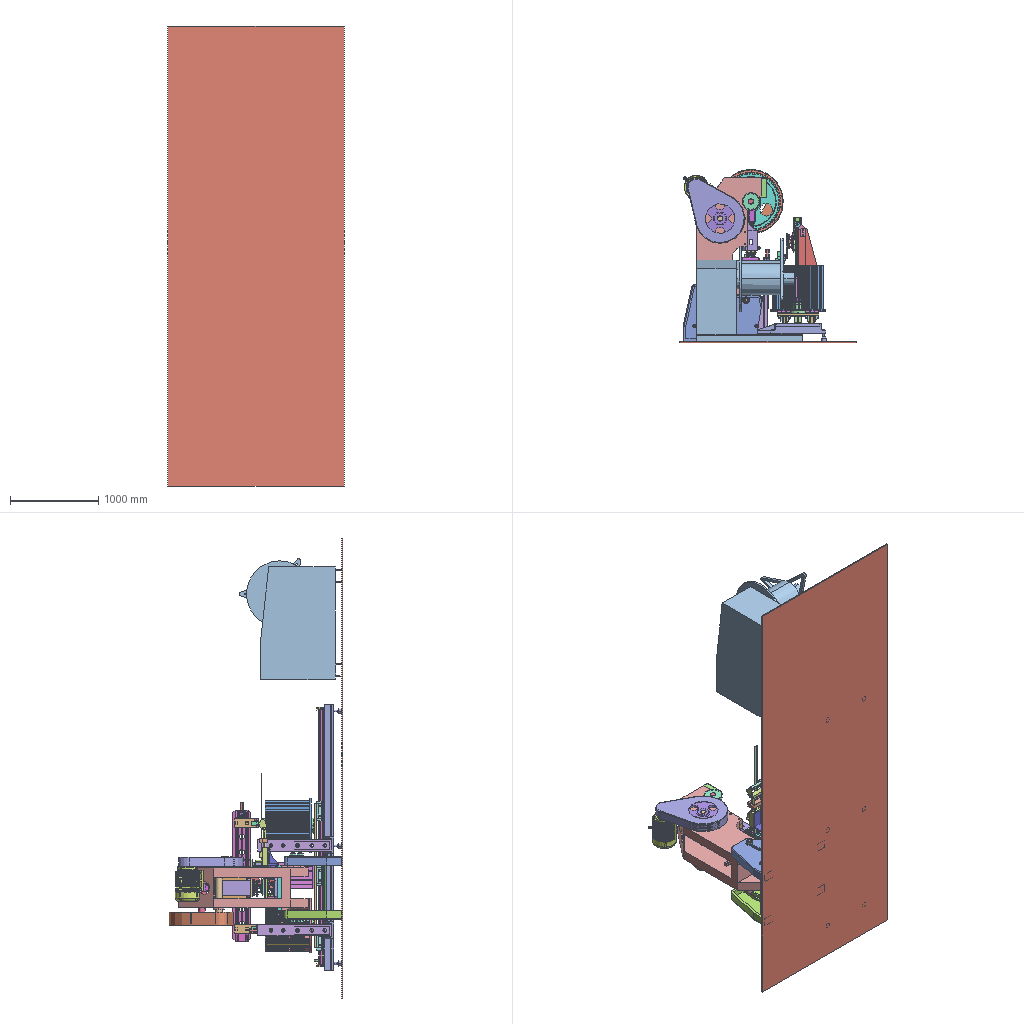Assembly | Creo | 143 different items | 263 placed | box 2000 x 1959 x 5200 mm
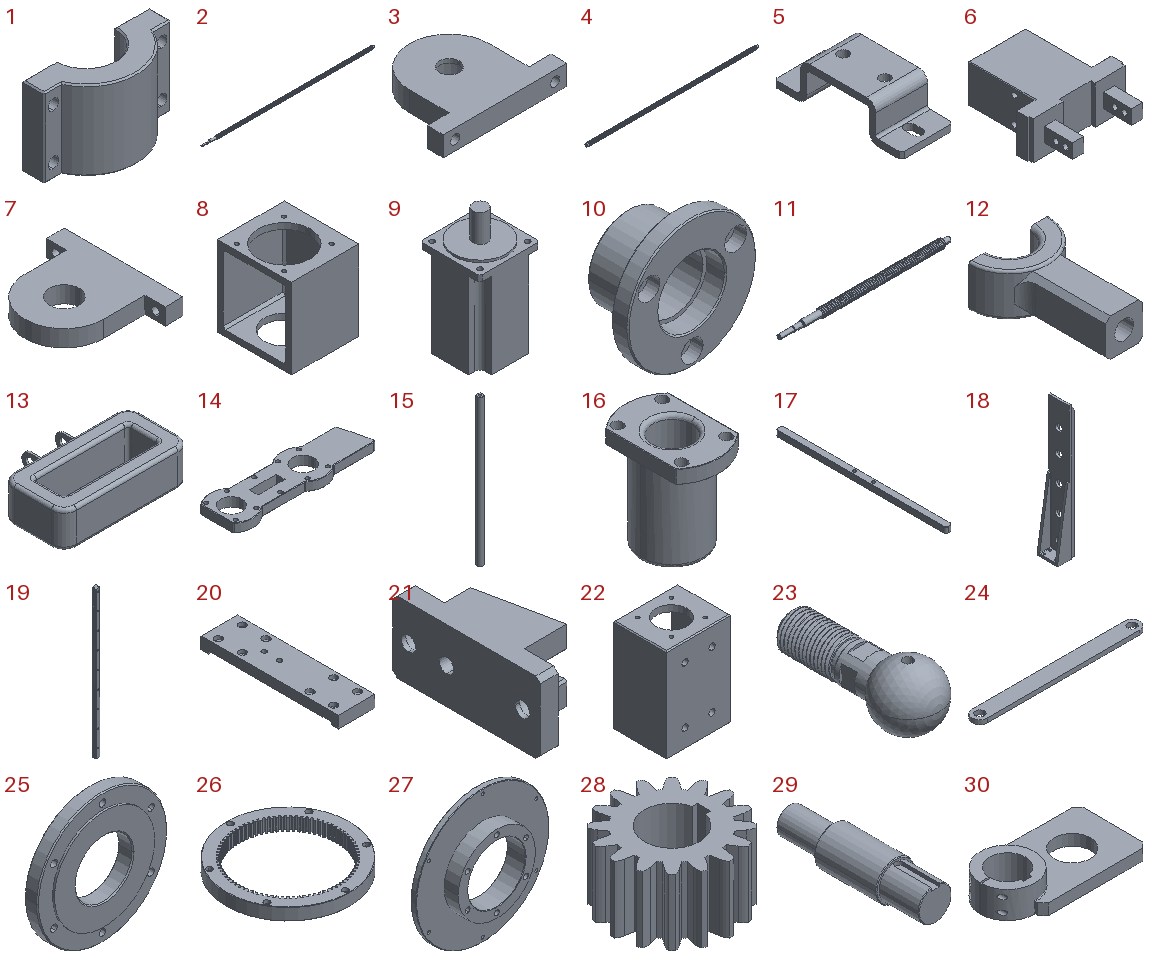Parts list (item | name | quantity | size | volume | features):
1 | - | x2 | 175.991 x 70 x 110 mm | 679965 mm3 | features DATUM PLANE 3, CURVE 2, CHAMFER 1, COORDINATE SYSTEM 1, CUT 1, PROTRUSION 1
2 | - | x1 | 712.5 x 12 x 12.001 mm | 63984 mm3 | features DATUM PLANE 3, COORDINATE SYSTEM 1, CURVE 1, CUT 1, PROTRUSION 1
3 | - | x1 | 62 x 48 x 10 mm | 16655 mm3 | features CURVE 4, CUT 3, DATUM PLANE 3, COORDINATE SYSTEM 1, PROTRUSION 1
4 | - | x1 | - | 61119 mm3 | features CURVE 3, CUT 3, DATUM PLANE 3, CHAMFER 1, COORDINATE SYSTEM 1, PROTRUSION 1
5 | - | x2 | 40 x 98 x 28.5 mm | 25930 mm3 | features DATUM PLANE 3, CURVE 2, ROUND 2, COORDINATE SYSTEM 1, CUT 1, PROTRUSION 1
6 | - | x2 | 119 x 139 x 48 mm | 401031 mm3 | features DATUM PLANE 3, CURVE 2, CHAMFER 1, COORDINATE SYSTEM 1, CUT 1, PROTRUSION 1
7 | - | x1 | 83 x 100 x 14 mm | 69421 mm3 | features DATUM PLANE 3, CURVE 2, COORDINATE SYSTEM 1, CUT 1, PROTRUSION 1
8 | - | x1 | 90 x 100 x 108 mm | 291545 mm3 | features CURVE 4, DATUM PLANE 3, CUT 2, PROTRUSION 2, CHAMFER 1, COORDINATE SYSTEM 1
9 | - | x2 | 80 x 80 x 162.2 mm | 703450 mm3 | features CURVE 4, DATUM PLANE 3, PROTRUSION 3, CHAMFER 1, COORDINATE SYSTEM 1, CUT 1
10 | - | x2 | 85.764 x 42.882 x 85.764 mm | 70979 mm3 | features CUT 4, CURVE 3, DATUM PLANE 3, CHAMFER 1, COORDINATE SYSTEM 1, PATTERN 1, PROTRUSION 1
11 | - | x1 | 414 x 20.009 x 20.003 mm | 92779 mm3 | features DATUM PLANE 3, COORDINATE SYSTEM 1, CURVE 1, CUT 1, PROTRUSION 1
12 | - | x1 | 170 x 245 x 90 mm | 1592709 mm3 | features CURVE 3, CUT 3, DATUM PLANE 3, ROUND 3, CHAMFER 1, COORDINATE SYSTEM 1, MIRROR 1, PROTRUSION 1
13 | - | x7 | 40 x 27.76 x 11.26 mm | 5415 mm3 | features CURVE 3, DATUM PLANE 3, PROTRUSION 2, ROUND 2, COORDINATE SYSTEM 1, CUT 1
14 | - | x1 | - | 47470 mm3 | features DATUM PLANE 3, CHAMFER 2, CURVE 2, COORDINATE SYSTEM 1, CUT 1, PROTRUSION 1, ROUND 1
15 | - | x12 | 20 x 20 x 500 mm | 128646 mm3 | features DATUM PLANE 3, CURVE 2, CHAMFER 1, COORDINATE SYSTEM 1, CUT 1, PROTRUSION 1
16 | - | x2 | 32 x 48 x 50 mm | 27898 mm3 | features DATUM PLANE 3, ROUND 3, CURVE 2, PROTRUSION 2, CHAMFER 1, COORDINATE SYSTEM 1
17 | - | x1 | 10 x 259.76 x 9 mm | 22836 mm3 | features DATUM PLANE 3, CHAMFER 1, COORDINATE SYSTEM 1, CURVE 1, PROTRUSION 1, ROUND 1
18 | - | x2 | 113.505 x 127.005 x 830 mm | 2691815 mm3 | features CURVE 5, PROTRUSION 4, DATUM PLANE 3, CUT 2, CHAMFER 1, COORDINATE SYSTEM 1, MIRROR 1
19 | - | x2 | - | 96624 mm3 | features CUT 12, CURVE 3, DATUM PLANE 3, COORDINATE SYSTEM 1, PATTERN 1, PROTRUSION 1
20 | - | x1 | 40 x 150 x 13 mm | 59155 mm3 | features CURVE 3, DATUM PLANE 3, PROTRUSION 2, COORDINATE SYSTEM 1, CUT 1
21 | - | x1 | 27.171 x 66.207 x 32 mm | 28820 mm3 | features CURVE 9, CUT 6, PROTRUSION 4, DATUM PLANE 3, CHAMFER 2, COORDINATE SYSTEM 1, MIRROR 1
22 | - | x1 | - | 99333 mm3 | features CURVE 10, CUT 6, DATUM PLANE 3, PROTRUSION 3, CHAMFER 2, COORDINATE SYSTEM 1
23 | - | x1 | 65 x 158.117 x 64.226 mm | 245084 mm3 | features CUT 7, CURVE 3, DATUM PLANE 3, CHAMFER 2, COORDINATE SYSTEM 1, PATTERN 1, PROTRUSION 1
24 | - | x6 | 194.76 x 18 x 5 mm | 16395 mm3 | features DATUM PLANE 3, COORDINATE SYSTEM 1, CURVE 1, PROTRUSION 1
25 | - | x2 | 130 x 15 x 130 mm | 144210 mm3 | features CUT 7, CURVE 3, DATUM PLANE 3, CHAMFER 1, COORDINATE SYSTEM 1, PATTERN 1, PROTRUSION 1
26 | - | x1 | 300 x 300 x 30 mm | 727858 mm3 | features PROTRUSION 81, CUT 7, CURVE 4, DATUM PLANE 3, PATTERN 2, CHAMFER 1, COORDINATE SYSTEM 1
27 | - | x1 | 300 x 44 x 300 mm | 925584 mm3 | features CURVE 7, CUT 6, DATUM PLANE 3, PATTERN 2, CHAMFER 1, COORDINATE SYSTEM 1, PROTRUSION 1
28 | - | x1 | 54 x 54 x 30 mm | 38517 mm3 | features PROTRUSION 17, DATUM PLANE 3, CURVE 2, COORDINATE SYSTEM 1, PATTERN 1
29 | - | x1 | 29 x 110.003 x 29 mm | 55617 mm3 | features DATUM PLANE 3, CURVE 2, CHAMFER 1, COORDINATE SYSTEM 1, CUT 1, PROTRUSION 1, ROUND 1
30 | - | x1 | 196.988 x 105 x 40 mm | 298699 mm3 | features CURVE 4, CUT 3, DATUM PLANE 3, CHAMFER 1, COORDINATE SYSTEM 1, PROTRUSION 1
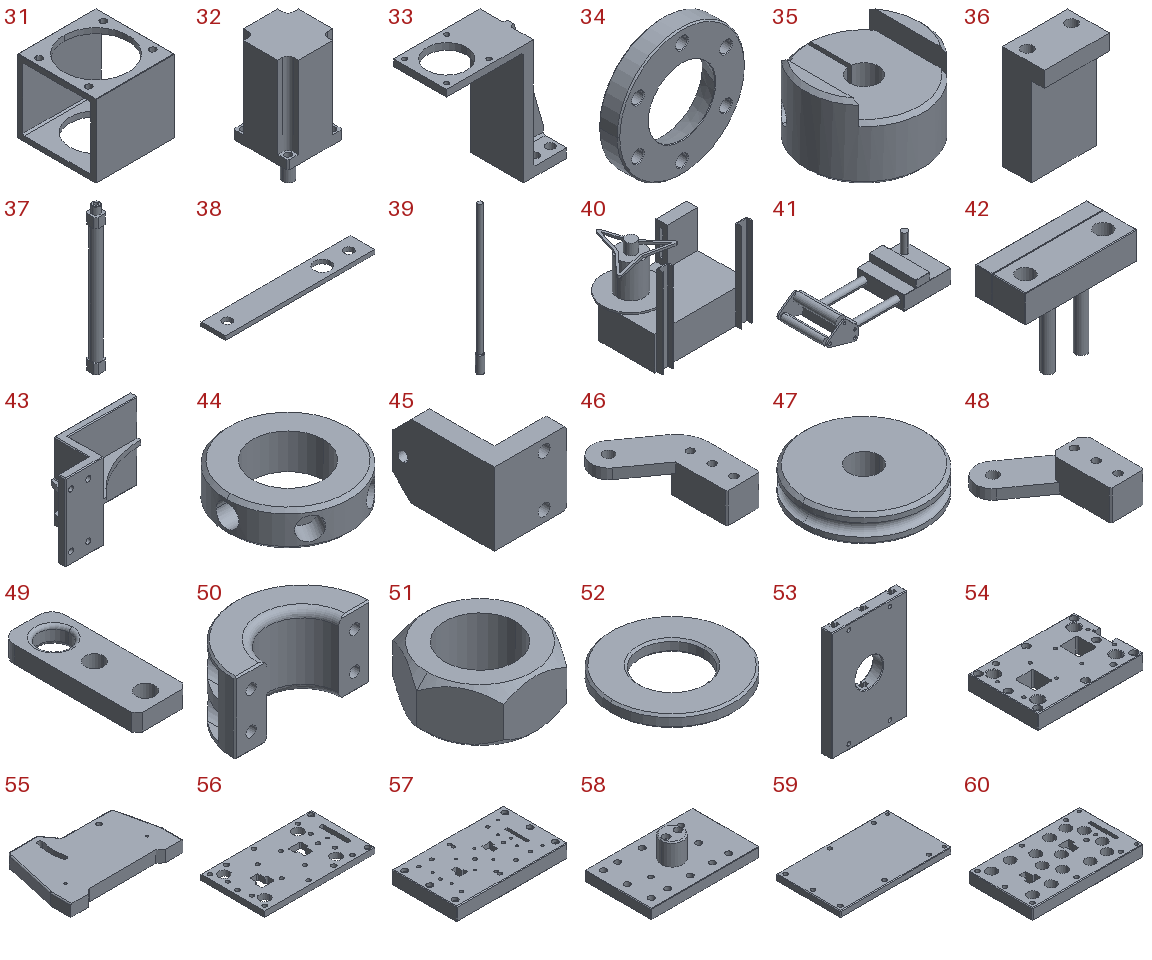31 | - | x1 | 105 x 105 x 98 mm | 209602 mm3 | features CURVE 3, DATUM PLANE 3, CHAMFER 2, CUT 2, COORDINATE SYSTEM 1, PROTRUSION 1
32 | - | x1 | 40 x 40 x 91.4 mm | 96010 mm3 | features CURVE 4, DATUM PLANE 3, PROTRUSION 3, CHAMFER 1, COORDINATE SYSTEM 1, CUT 1
33 | - | x1 | 90 x 40 x 90 mm | 46256 mm3 | features CURVE 6, PROTRUSION 4, DATUM PLANE 3, CUT 2, CHAMFER 1, COORDINATE SYSTEM 1
34 | - | x1 | 95 x 15 x 95 mm | 60557 mm3 | features CUT 7, CURVE 3, DATUM PLANE 3, CHAMFER 2, COORDINATE SYSTEM 1, PATTERN 1, PROTRUSION 1
35 | - | x1 | - | 11116 mm3 | features CURVE 3, DATUM PLANE 3, CUT 2, CHAMFER 1, COORDINATE SYSTEM 1, PROTRUSION 1
36 | - | x4 | 50 x 32 x 80 mm | 84921 mm3 | features DATUM PLANE 3, CURVE 2, PROTRUSION 2, COORDINATE SYSTEM 1
37 | - | x2 | - | 15001 mm3 | features CURVE 3, DATUM PLANE 3, PROTRUSION 2, CHAMFER 1, COORDINATE SYSTEM 1, CUT 1
38 | - | x2 | 74 x 12 x 2 mm | 1612 mm3 | features DATUM PLANE 3, COORDINATE SYSTEM 1, CURVE 1, PROTRUSION 1
39 | - | x2 | 6 x 6 x 136 mm | 1956 mm3 | features DATUM PLANE 3, CURVE 2, PROTRUSION 2, CHAMFER 1, COORDINATE SYSTEM 1
40 | - | x1 | - | 559581150 mm3 | features CURVE 11, PROTRUSION 10, CUT 4, DATUM PLANE 3, ROUND 2, COORDINATE SYSTEM 1, MIRROR 1, PATTERN 1
41 | - | x1 | 534.884 x 212 x 140 mm | 3889632 mm3 | features PROTRUSION 8, CURVE 7, DATUM PLANE 3, CHAMFER 2, COORDINATE SYSTEM 1, MIRROR 1
42 | - | x1 | 200 x 90 x 170 mm | 903544 mm3 | features CURVE 3, DATUM PLANE 3, PROTRUSION 3, CHAMFER 2, COORDINATE SYSTEM 1
43 | - | x1 | 280 x 110 x 200 mm | 1505598 mm3 | features CURVE 3, DATUM PLANE 3, CHAMFER 2, PROTRUSION 2, COORDINATE SYSTEM 1, CUT 1
44 | - | x1 | 70 x 70 x 20 mm | 41537 mm3 | features CUT 6, DATUM PLANE 4, CURVE 2, CHAMFER 1, COORDINATE SYSTEM 1, PATTERN 1, PROTRUSION 1
45 | - | x1 | 80 x 111 x 80 mm | 282107 mm3 | features CURVE 4, DATUM PLANE 3, CHAMFER 2, CUT 2, PROTRUSION 2, COORDINATE SYSTEM 1
46 | - | x1 | 115 x 160.005 x 45 mm | 256646 mm3 | features DATUM PLANE 3, CURVE 2, PROTRUSION 2, CHAMFER 1, COORDINATE SYSTEM 1
47 | - | x2 | 80 x 80 x 18 mm | 77786 mm3 | features DATUM PLANE 3, CHAMFER 1, COORDINATE SYSTEM 1, CURVE 1, CUT 1, PROTRUSION 1
48 | - | x1 | 115 x 160.005 x 45 mm | 256646 mm3 | features DATUM PLANE 3, CURVE 2, PROTRUSION 2, CHAMFER 1, COORDINATE SYSTEM 1
49 | - | x2 | 30 x 80 x 10 mm | 19088 mm3 | features DATUM PLANE 3, CHAMFER 1, COORDINATE SYSTEM 1, CURVE 1, PROTRUSION 1, ROUND 1
50 | - | x1 | 170 x 85 x 90 mm | 620159 mm3 | features DATUM PLANE 4, CURVE 3, CUT 2, CHAMFER 1, COORDINATE SYSTEM 1, PROTRUSION 1, ROUND 1
51 | - | x2 | - | 4002 mm3 | features DATUM PLANE 3, CURVE 2, CHAMFER 1, COORDINATE SYSTEM 1, CUT 1, PROTRUSION 1
52 | - | x2 | 31 x 31 x 3 mm | 1624 mm3 | features DATUM PLANE 3, CHAMFER 1, COORDINATE SYSTEM 1, CURVE 1, PROTRUSION 1
53 | - | x1 | 349.97 x 50 x 510 mm | 7245809 mm3 | features CURVE 3, DATUM PLANE 3, CUT 2, CHAMFER 1, COORDINATE SYSTEM 1, PROTRUSION 1
54 | - | x1 | 157.5 x 103.5 x 22.5 mm | 294223 mm3 | features DATUM PLANE 3, CURVE 2, CHAMFER 1, COORDINATE SYSTEM 1, CUT 1, PROTRUSION 1, ROUND 1
55 | - | x1 | 960 x 650 x 100 mm | 16944172 mm3 | features CURVE 6, PROTRUSION 4, DATUM PLANE 3, ROUND 3, COORDINATE SYSTEM 1, CUT 1
56 | - | x1 | 179.25 x 103.5 x 9 mm | 143240 mm3 | features DATUM PLANE 3, CURVE 2, COORDINATE SYSTEM 1, CUT 1, PROTRUSION 1
57 | - | x1 | 229.25 x 133.5 x 28 mm | 806588 mm3 | features CURVE 4, CUT 3, DATUM PLANE 3, CHAMFER 1, COORDINATE SYSTEM 1, PROTRUSION 1
58 | - | x1 | 199.25 x 123.5 x 58 mm | 470509 mm3 | features CURVE 4, DATUM PLANE 3, CHAMFER 2, CUT 2, PROTRUSION 2, COORDINATE SYSTEM 1
59 | - | x1 | 179.25 x 103.5 x 10 mm | 182337 mm3 | features DATUM PLANE 3, CHAMFER 1, COORDINATE SYSTEM 1, CURVE 1, PROTRUSION 1
60 | - | x1 | 179.25 x 103.5 x 18 mm | 263298 mm3 | features DATUM PLANE 3, CHAMFER 1, COORDINATE SYSTEM 1, CURVE 1, PROTRUSION 1
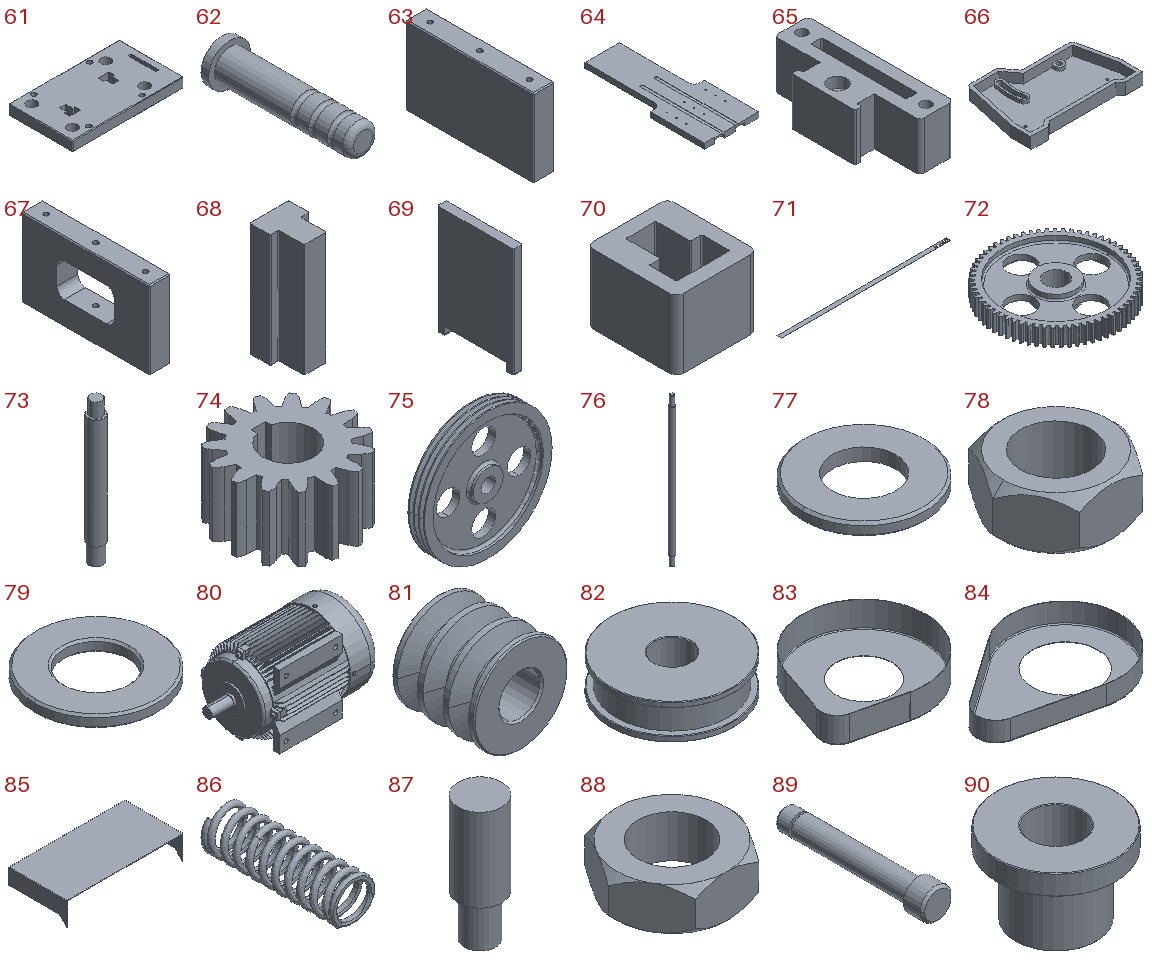61 | - | x1 | 179.25 x 103.5 x 16 mm | 267287 mm3 | features DATUM PLANE 3, CURVE 2, PROTRUSION 2, CHAMFER 1, COORDINATE SYSTEM 1
62 | - | x4 | 22 x 74 x 22 mm | 15015 mm3 | features DATUM PLANE 3, COORDINATE SYSTEM 1, CURVE 1, PROTRUSION 1
63 | - | x2 | 22 x 133.5 x 82 mm | 235535 mm3 | features DATUM PLANE 3, CHAMFER 1, COORDINATE SYSTEM 1, CURVE 1, PROTRUSION 1
64 | - | x1 | 289.25 x 690 x 28 mm | 4080751 mm3 | features CURVE 9, CUT 5, PROTRUSION 4, DATUM PLANE 3, ROUND 3, COORDINATE SYSTEM 1
65 | - | x1 | 27 x 68.5 x 22.5 mm | 24185 mm3 | features DATUM PLANE 3, CURVE 2, COORDINATE SYSTEM 1, CUT 1, PROTRUSION 1, ROUND 1
66 | - | x1 | 960 x 650 x 100 mm | 16944172 mm3 | features CURVE 5, PROTRUSION 4, ROUND 4, DATUM PLANE 3, COORDINATE SYSTEM 1, CUT 1
67 | - | x1 | 22 x 133.5 x 82 mm | 191231 mm3 | features DATUM PLANE 3, CURVE 2, CHAMFER 1, COORDINATE SYSTEM 1, CUT 1, PROTRUSION 1, ROUND 1
68 | - | x2 | 17.25 x 20.25 x 52 mm | 13253 mm3 | features DATUM PLANE 3, CURVE 2, PROTRUSION 2, CHAMFER 1, COORDINATE SYSTEM 1
69 | - | x1 | 5.25 x 45 x 65 mm | 14350 mm3 | features DATUM PLANE 3, CURVE 2, COORDINATE SYSTEM 1, CUT 1, PROTRUSION 1, ROUND 1
70 | - | x2 | 26.25 x 29.25 x 22.5 mm | 11220 mm3 | features DATUM PLANE 3, COORDINATE SYSTEM 1, CURVE 1, PROTRUSION 1
71 | - | x1 | 1347 x 36.003 x 0.5 mm | 23317 mm3 | features DATUM PLANE 3, CURVE 2, PROTRUSION 2, COORDINATE SYSTEM 1
72 | - | x1 | 669.936 x 669.757 x 90 mm | 13299153 mm3 | features PROTRUSION 66, CURVE 5, CUT 3, DATUM PLANE 3, COORDINATE SYSTEM 1, PATTERN 1, ROUND 1
73 | - | x1 | 80 x 80 x 717 mm | 3328283 mm3 | features CURVE 4, CUT 3, DATUM PLANE 3, CHAMFER 1, COORDINATE SYSTEM 1, PROTRUSION 1, ROUND 1
74 | - | x1 | 169.638 x 168.774 x 90 mm | 1195621 mm3 | features PROTRUSION 16, CURVE 3, DATUM PLANE 3, COORDINATE SYSTEM 1, CUT 1, PATTERN 1
75 | - | x1 | 540 x 70.006 x 540 mm | 7681401 mm3 | features CUT 4, DATUM PLANE 3, CURVE 2, COORDINATE SYSTEM 1, PATTERN 1, PROTRUSION 1
76 | - | x2 | 28 x 28 x 770 mm | 443735 mm3 | features DATUM PLANE 3, CURVE 2, PROTRUSION 2, CHAMFER 1, COORDINATE SYSTEM 1
77 | - | x4 | 78 x 78 x 8 mm | 27630 mm3 | features DATUM PLANE 3, CHAMFER 1, COORDINATE SYSTEM 1, CURVE 1, PROTRUSION 1
78 | - | x4 | - | 7816 mm3 | features DATUM PLANE 3, CURVE 2, CHAMFER 1, COORDINATE SYSTEM 1, CUT 1, PROTRUSION 1
79 | - | x4 | 38.75 x 38.75 x 3.75 mm | 3172 mm3 | features DATUM PLANE 3, CHAMFER 1, COORDINATE SYSTEM 1, CURVE 1, PROTRUSION 1
80 | - | x1 | 477.5 x 323.125 x 283.75 mm | 16550696 mm3 | features COORDINATE SYSTEM 1, IMPORT FEATURE 1
81 | - | x1 | 80 x 70 x 80 mm | 169146 mm3 | features DATUM PLANE 3, CHAMFER 2, COORDINATE SYSTEM 1, CURVE 1, PROTRUSION 1
82 | - | x1 | 200 x 200 x 57 mm | 1403837 mm3 | features DATUM PLANE 3, CHAMFER 1, COORDINATE SYSTEM 1, CURVE 1, CUT 1, PROTRUSION 1
83 | - | x1 | 813.936 x 730.395 x 152 mm | 1449913 mm3 | features DATUM PLANE 3, CURVE 2, PROTRUSION 2, ROUND 2, COORDINATE SYSTEM 1
84 | - | x1 | 814.237 x 560 x 102 mm | 885224 mm3 | features DATUM PLANE 3, CURVE 2, PROTRUSION 2, ROUND 2, COORDINATE SYSTEM 1
85 | - | x1 | 450 x 225 x 92 mm | 311820 mm3 | features PROTRUSION 5, CURVE 4, DATUM PLANE 3, COORDINATE SYSTEM 1, MIRROR 1
86 | - | x4 | - | 1308 mm3 | features DATUM PLANE 4, PROTRUSION 3, CURVE 2, CUT 2, COORDINATE SYSTEM 1
87 | - | x4 | 10.5 x 10.5 x 30 mm | 2174 mm3 | features DATUM PLANE 3, CURVE 2, PROTRUSION 2, COORDINATE SYSTEM 1
88 | - | x4 | - | 58909 mm3 | features DATUM PLANE 3, CURVE 2, CHAMFER 1, COORDINATE SYSTEM 1, CUT 1, PROTRUSION 1
89 | - | x8 | 6.5 x 32 x 6.5 mm | 570.854 mm3 | features DATUM PLANE 3, COORDINATE SYSTEM 1, CURVE 1, PROTRUSION 1
90 | - | x1 | 176 x 176 x 120 mm | 1202377 mm3 | features DATUM PLANE 3, CURVE 2, PROTRUSION 2, CHAMFER 1, COORDINATE SYSTEM 1
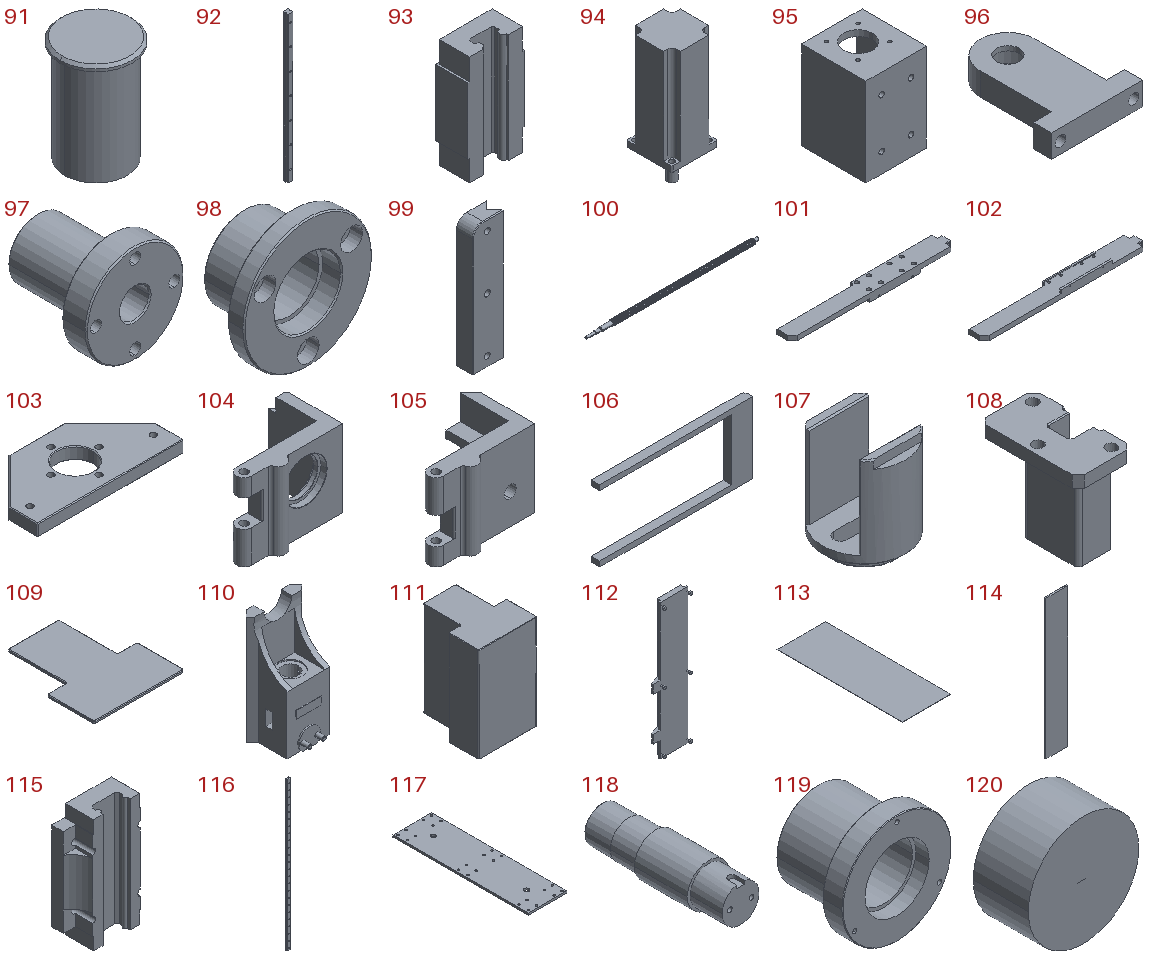91 | - | x1 | 58 x 58 x 84 mm | 167292 mm3 | features DATUM PLANE 3, CURVE 2, PROTRUSION 2, CHAMFER 1, COORDINATE SYSTEM 1
92 | - | x2 | 14.99 x 14 x 412 mm | 76604 mm3 | features CUT 8, CURVE 3, DATUM PLANE 3, COORDINATE SYSTEM 1, PATTERN 1, PROTRUSION 1
93 | - | x10 | 34 x 19.4 x 66 mm | 33141 mm3 | features CURVE 3, DATUM PLANE 3, PROTRUSION 2, COORDINATE SYSTEM 1, CUT 1
94 | - | x4 | 40 x 40 x 114 mm | 127179 mm3 | features CURVE 4, DATUM PLANE 3, PROTRUSION 3, CHAMFER 1, COORDINATE SYSTEM 1, CUT 1
95 | - | x1 | 62 x 66 x 90.5 mm | 126268 mm3 | features CURVE 7, CUT 4, DATUM PLANE 3, PROTRUSION 2, CHAMFER 1, COORDINATE SYSTEM 1
96 | - | x1 | 40 x 51 x 10 mm | 10314 mm3 | features CURVE 4, CUT 3, DATUM PLANE 3, COORDINATE SYSTEM 1, PROTRUSION 1
97 | - | x2 | 40 x 40 x 40 mm | 20928 mm3 | features DATUM PLANE 3, CURVE 2, CHAMFER 1, COORDINATE SYSTEM 1, CUT 1, PROTRUSION 1
98 | - | x3 | 54 x 27 x 54 mm | 17717 mm3 | features CUT 4, CURVE 3, DATUM PLANE 3, CHAMFER 1, COORDINATE SYSTEM 1, PATTERN 1, PROTRUSION 1
99 | - | x2 | 90 x 50 x 380 mm | 1426529 mm3 | features DATUM PLANE 3, CURVE 2, CHAMFER 1, COORDINATE SYSTEM 1, CUT 1, PROTRUSION 1, ROUND 1
100 | - | x1 | 399.5 x 12 x 12.003 mm | 34208 mm3 | features DATUM PLANE 3, COORDINATE SYSTEM 1, CURVE 1, CUT 1, PROTRUSION 1
101 | - | x1 | 350.982 x 41 x 17 mm | 128425 mm3 | features CURVE 6, CUT 3, DATUM PLANE 3, PROTRUSION 3, COORDINATE SYSTEM 1
102 | - | x1 | 350.982 x 41 x 17 mm | 128458 mm3 | features CURVE 6, CUT 3, DATUM PLANE 3, PROTRUSION 3, COORDINATE SYSTEM 1
103 | - | x1 | 97 x 49 x 8 mm | 26205 mm3 | features DATUM PLANE 3, CURVE 2, CHAMFER 1, COORDINATE SYSTEM 1, CUT 1, PROTRUSION 1
104 | - | x1 | 65 x 47 x 51 mm | 35916 mm3 | features CURVE 9, CUT 5, PROTRUSION 4, DATUM PLANE 3, ROUND 3, CHAMFER 2, COORDINATE SYSTEM 1
105 | - | x1 | 65 x 47 x 51 mm | 44748 mm3 | features CURVE 7, PROTRUSION 5, DATUM PLANE 3, ROUND 3, CUT 2, CHAMFER 1, COORDINATE SYSTEM 1
106 | - | x1 | - | 184057 mm3 | features CURVE 3, DATUM PLANE 3, PROTRUSION 2, COORDINATE SYSTEM 1, CUT 1, ROUND 1
107 | - | x1 | 30 x 30 x 36 mm | 8414 mm3 | features CURVE 5, CHAMFER 3, DATUM PLANE 3, PROTRUSION 3, CUT 2, COORDINATE SYSTEM 1
108 | - | x1 | - | 19348 mm3 | features CURVE 3, DATUM PLANE 3, CHAMFER 2, CUT 2, COORDINATE SYSTEM 1, PROTRUSION 1, ROUND 1
109 | - | x8 | 17.25 x 20.25 x 0.5 mm | 131.673 mm3 | features DATUM PLANE 3, CHAMFER 1, COORDINATE SYSTEM 1, CURVE 1, PROTRUSION 1
110 | - | x1 | - | 7776005 mm3 | features CURVE 11, CUT 7, PROTRUSION 4, DATUM PLANE 3, CHAMFER 1, COORDINATE SYSTEM 1
111 | - | x2 | 17.25 x 20.25 x 28 mm | 7414 mm3 | features DATUM PLANE 3, CHAMFER 1, COORDINATE SYSTEM 1, CURVE 1, PROTRUSION 1
112 | - | x1 | 780 x 200 x 3010 mm | 141202284 mm3 | features PROTRUSION 8, CURVE 6, CHAMFER 3, DATUM PLANE 3, MOVE 2, COORDINATE SYSTEM 1, CUT 1
113 | - | x1 | 2000 x 5200 x 10 mm | 104000000 mm3 | features DATUM PLANE 3, COORDINATE SYSTEM 1, CURVE 1, PROTRUSION 1
114 | - | x1 | - | 47662635 mm3 | features DATUM PLANE 3, CHAMFER 2, CURVE 2, COORDINATE SYSTEM 1, CUT 1, PROTRUSION 1
115 | - | x6 | 140 x 57.3 x 223 mm | 1103476 mm3 | features CURVE 5, CUT 3, DATUM PLANE 3, PROTRUSION 3, COORDINATE SYSTEM 1, MIRROR 1
116 | - | x2 | 53 x 38 x 2870 mm | 5298046 mm3 | features CUT 48, CURVE 3, DATUM PLANE 3, PATTERN 2, CHAMFER 1, COORDINATE SYSTEM 1, PROTRUSION 1
117 | - | x1 | 468 x 1636 x 24 mm | 15910357 mm3 | features CURVE 4, DATUM PLANE 3, CUT 2, PROTRUSION 2, COORDINATE SYSTEM 1
118 | - | x2 | 63 x 207 x 63 mm | 538565 mm3 | features CURVE 3, DATUM PLANE 3, CUT 2, ROUND 2, CHAMFER 1, COORDINATE SYSTEM 1, PROTRUSION 1
119 | - | x2 | 170 x 123 x 170 mm | 1070744 mm3 | features CUT 9, CURVE 3, DATUM PLANE 3, PATTERN 2, CHAMFER 1, COORDINATE SYSTEM 1, PROTRUSION 1
120 | - | x1 | 65 x 32.5 x 65 mm | 35948 mm3 | features DATUM PLANE 3, COORDINATE SYSTEM 1, CURVE 1, PROTRUSION 1
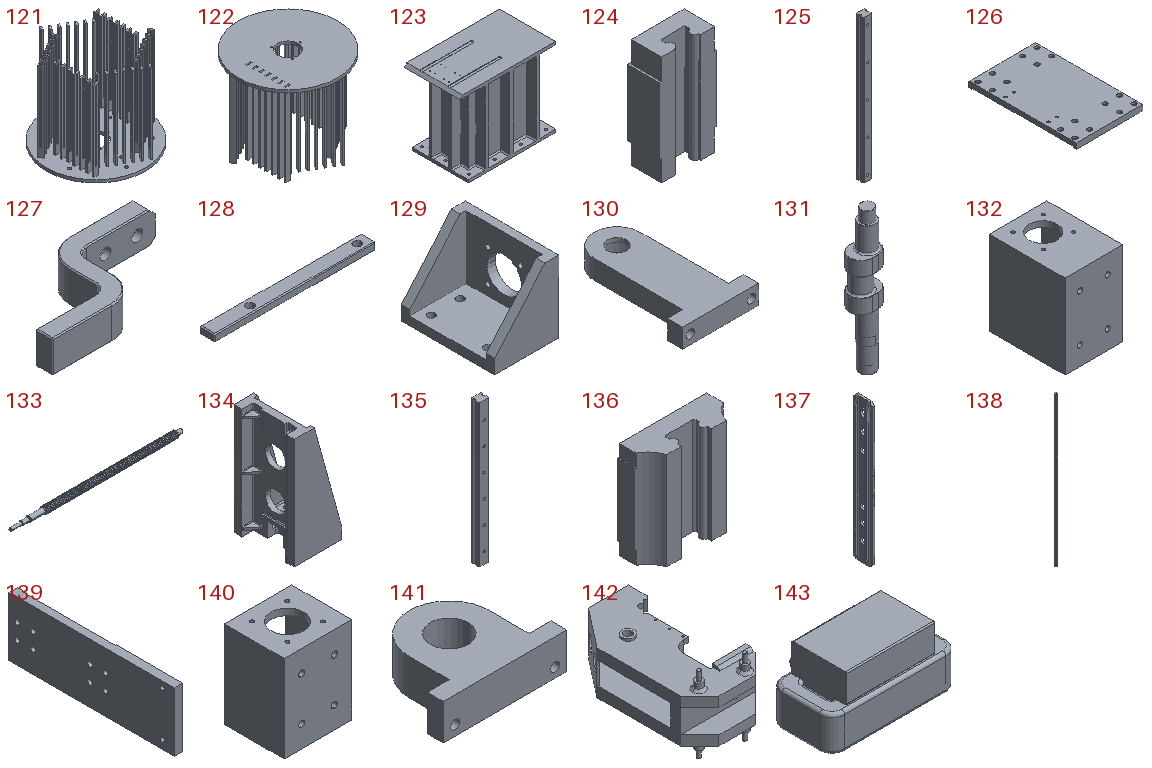121 | - | x1 | 620 x 620 x 518 mm | 9371630 mm3 | features CUT 12, PROTRUSION 7, CURVE 4, DATUM PLANE 3, PATTERN 3, COORDINATE SYSTEM 1
122 | - | x1 | 620 x 620 x 518 mm | 11304252 mm3 | features PROTRUSION 7, DATUM PLANE 3, CURVE 2, COORDINATE SYSTEM 1, PATTERN 1
123 | - | x1 | 512 x 300 x 421 mm | 36405249 mm3 | features CUT 7, CURVE 6, DATUM PLANE 3, MOVE 3, CHAMFER 2, PROTRUSION 2, COORDINATE SYSTEM 1, ROUND 1
124 | - | x4 | 34 x 19.41 x 66 mm | 33431 mm3 | features CURVE 3, DATUM PLANE 3, PROTRUSION 2, COORDINATE SYSTEM 1, CUT 1
125 | - | x2 | 15 x 14 x 265 mm | 47944 mm3 | features CUT 6, CURVE 3, DATUM PLANE 3, COORDINATE SYSTEM 1, PATTERN 1, PROTRUSION 1
126 | - | x1 | 120 x 192 x 10 mm | 182173 mm3 | features CURVE 3, DATUM PLANE 3, PROTRUSION 2, COORDINATE SYSTEM 1, CUT 1
127 | - | x2 | 78.5 x 38 x 15.3 mm | 11414 mm3 | features CURVE 3, DATUM PLANE 3, CHAMFER 2, CUT 2, COORDINATE SYSTEM 1, PROTRUSION 1
128 | - | x4 | 87 x 8 x 4 mm | 2624 mm3 | features DATUM PLANE 3, CHAMFER 1, COORDINATE SYSTEM 1, CURVE 1, PROTRUSION 1
129 | - | x1 | - | 43444 mm3 | features CURVE 4, CUT 3, DATUM PLANE 3, CHAMFER 1, COORDINATE SYSTEM 1, PROTRUSION 1
130 | - | x1 | 40 x 66.5 x 10 mm | 14034 mm3 | features CURVE 4, CUT 3, DATUM PLANE 3, COORDINATE SYSTEM 1, PROTRUSION 1
131 | - | x1 | 140 x 110 x 687 mm | 4490252 mm3 | features PROTRUSION 9, CURVE 8, DATUM PLANE 3, CHAMFER 2, MIRROR 2, ROUND 2, COORDINATE SYSTEM 1, CUT 1
132 | - | x1 | 62 x 81.5 x 90.5 mm | 211765 mm3 | features CURVE 7, CUT 4, DATUM PLANE 3, PROTRUSION 2, CHAMFER 1, COORDINATE SYSTEM 1
133 | - | x1 | 310.5 x 12.006 x 12.001 mm | 25764 mm3 | features DATUM PLANE 3, COORDINATE SYSTEM 1, CURVE 1, CUT 1, PROTRUSION 1
134 | - | x1 | 240.512 x 299.995 x 550 mm | 9242753 mm3 | features CURVE 9, PROTRUSION 8, CUT 6, DATUM PLANE 3, CHAMFER 2, MOVE 2, COORDINATE SYSTEM 1, MIRROR 1, ROUND 1
135 | - | x2 | 33.99 x 29 x 500 mm | 443618 mm3 | features CUT 7, CURVE 3, DATUM PLANE 3, COORDINATE SYSTEM 1, PATTERN 1, PROTRUSION 1
136 | - | x4 | 100 x 38.5 x 109 mm | 303795 mm3 | features CURVE 3, DATUM PLANE 3, PROTRUSION 2, COORDINATE SYSTEM 1, CUT 1
137 | - | x1 | 53 x 205 x 1480 mm | 7789168 mm3 | features CURVE 12, CUT 10, DATUM PLANE 3, PROTRUSION 3, ROUND 3, CHAMFER 1, COORDINATE SYSTEM 1, MIRROR 1
138 | - | x2 | 14.99 x 14 x 1320 mm | 245585 mm3 | features CUT 23, CURVE 3, DATUM PLANE 3, COORDINATE SYSTEM 1, PATTERN 1, PROTRUSION 1
139 | - | x2 | 14 x 273.995 x 98 mm | 341996 mm3 | features CURVE 5, CUT 3, DATUM PLANE 3, PROTRUSION 2, COORDINATE SYSTEM 1
140 | - | x1 | 62 x 55 x 80 mm | 96326 mm3 | features CURVE 6, CUT 4, DATUM PLANE 3, PROTRUSION 2, CHAMFER 1, COORDINATE SYSTEM 1
141 | - | x1 | 62 x 48 x 18 mm | 29280 mm3 | features CURVE 3, DATUM PLANE 3, CUT 2, COORDINATE SYSTEM 1, PROTRUSION 1
142 | - | x1 | 780 x 1470 x 790 mm | 186494626 mm3 | features CURVE 13, PROTRUSION 10, CUT 7, CHAMFER 3, DATUM PLANE 3, MIRROR 3, COORDINATE SYSTEM 1
143 | (subassembly) | x1 | 40 x 27.76 x 20.26 mm | 12829 mm3 | features DATUM PLANE 3, COMPONENT 2, COORDINATE SYSTEM 1
Mates (type | each side: item.copy, entity, surface, feature), first 229 of 577 lines:
ASM_CONSTRAINT_ALIGN | assembly plane datum plane | 142.1 plane datum plane | 3 times
ASM_CONSTRAINT_MATE | 142.1 face plane protrusion | 55.1 face plane protrusion
ASM_CONSTRAINT_INSERT | 142.1 face cylinder protrusion | 55.1 face cylinder protrusion
ASM_CONSTRAINT_ALIGN_ANG_OFF | 142.1 face plane protrusion | 55.1 face plane protrusion
ASM_CONSTRAINT_MATE_OFF | 142.1 face plane protrusion | 66.1 face plane protrusion
ASM_CONSTRAINT_INSERT | 142.1 face cylinder protrusion | 66.1 face cylinder protrusion
ASM_CONSTRAINT_MATE_ANG_OFF | 142.1 face plane protrusion | 66.1 face plane protrusion
ASM_CONSTRAINT_MATE_OFF | 55.1 face plane protrusion | 77.1 face plane protrusion
ASM_CONSTRAINT_INSERT | 142.1 face cylinder protrusion | 77.1 face cylinder protrusion
ASM_CONSTRAINT_MATE | 55.1 face plane protrusion | 77.2 face plane protrusion
ASM_CONSTRAINT_INSERT | 142.1 face cylinder protrusion | 77.2 face cylinder protrusion
ASM_CONSTRAINT_MATE_OFF | 66.1 face plane protrusion | 77.3 face plane protrusion
ASM_CONSTRAINT_INSERT | 142.1 face cylinder protrusion | 77.3 face cylinder protrusion
ASM_CONSTRAINT_MATE_OFF | 66.1 face plane protrusion | 77.4 face plane protrusion
ASM_CONSTRAINT_INSERT | 142.1 face cylinder protrusion | 77.4 face cylinder protrusion
ASM_CONSTRAINT_INSERT | 142.1 face cylinder protrusion | 88.1 face cylinder protrusion
ASM_CONSTRAINT_MATE | 77.1 face plane protrusion | 88.1 face plane protrusion
ASM_CONSTRAINT_MATE | 77.2 face plane protrusion | 88.2 face plane protrusion
ASM_CONSTRAINT_INSERT | 142.1 face cylinder protrusion | 88.2 face cylinder protrusion
ASM_CONSTRAINT_MATE_OFF | 77.3 face plane protrusion | 88.3 face plane protrusion
ASM_CONSTRAINT_INSERT | 142.1 face cylinder protrusion | 88.3 face cylinder protrusion
ASM_CONSTRAINT_MATE_OFF | 77.4 face plane protrusion | 88.4 face plane protrusion
ASM_CONSTRAINT_INSERT | 142.1 face cylinder protrusion | 88.4 face cylinder protrusion
ASM_CONSTRAINT_MATE_OFF | 142.1 face plane cut | 99.1 face plane protrusion | 2 times
ASM_CONSTRAINT_MATE | 142.1 face plane cut | 99.1 face plane protrusion
ASM_CONSTRAINT_MATE | 142.1 face plane cut | 99.2 face plane protrusion
ASM_CONSTRAINT_MATE_OFF | 142.1 face plane cut | 99.2 face plane protrusion | 2 times
ASM_CONSTRAINT_MATE | 99.2 face plane protrusion | 110.1 face plane protrusion | 2 times
ASM_CONSTRAINT_MATE_OFF | 110.1 face plane cut | 120.1 face plane protrusion
ASM_CONSTRAINT_INSERT | 110.1 face cylinder cut | 120.1 face cylinder protrusion
ASM_CONSTRAINT_INSERT | 142.1 face cylinder protrusion | 131.1 face cylinder protrusion
ASM_CONSTRAINT_MATE | 142.1 face plane cut | 131.1 face plane protrusion
ASM_CONSTRAINT_MATE_OFF | 142.1 face plane protrusion | 1.1 face plane protrusion | 2 times
ASM_CONSTRAINT_ALIGN_OFF | 142.1 face plane protrusion | 1.1 face plane protrusion
ASM_CONSTRAINT_MATE_OFF | 142.1 face plane protrusion | 1.2 face plane protrusion | 2 times
ASM_CONSTRAINT_ALIGN_OFF | 142.1 face plane cut | 1.2 face plane protrusion
ASM_CONSTRAINT_INSERT | 110.1 face cylinder cut | 23.1 face cylinder cut
ASM_CONSTRAINT_MATE | 110.1 plane datum plane | 23.1 plane datum plane
ASM_CONSTRAINT_INSERT | 23.1 face cylinder protrusion | 12.1 face cylinder cut
ASM_CONSTRAINT_MATE | 23.1 face plane protrusion | 12.1 face plane protrusion
ASM_CONSTRAINT_INSERT | 131.1 face cylinder protrusion | 12.1 face cylinder protrusion
ASM_CONSTRAINT_MATE_OFF | 110.1 face plane cut | 34.1 face plane protrusion
ASM_CONSTRAINT_INSERT | 110.1 face cylinder cut | 34.1 face cylinder protrusion
ASM_CONSTRAINT_MATE_OFF | 12.1 face plane protrusion | 44.1 face plane protrusion
ASM_CONSTRAINT_INSERT | 12.1 face cylinder cut | 44.1 face cylinder protrusion
ASM_CONSTRAINT_MATE_OFF | 12.1 face plane protrusion | 50.1 face plane protrusion
ASM_CONSTRAINT_INSERT | 131.1 face cylinder protrusion | 50.1 face cylinder protrusion
ASM_CONSTRAINT_MATE_OFF | 131.1 face plane protrusion | 50.1 face plane protrusion
ASM_CONSTRAINT_MATE_OFF | 110.1 face plane protrusion | 51.1 face plane protrusion
ASM_CONSTRAINT_INSERT | 110.1 face cylinder protrusion | 51.1 face cylinder protrusion
ASM_CONSTRAINT_MATE_OFF | 110.1 face plane protrusion | 51.2 face plane protrusion
ASM_CONSTRAINT_INSERT | 110.1 face cylinder protrusion | 51.2 face cylinder protrusion
ASM_CONSTRAINT_MATE_OFF | 110.1 face plane protrusion | 52.1 face plane protrusion
ASM_CONSTRAINT_INSERT | 110.1 face cylinder protrusion | 52.1 face cylinder protrusion
ASM_CONSTRAINT_MATE_OFF | 110.1 face plane protrusion | 52.2 face plane protrusion
ASM_CONSTRAINT_INSERT | 110.1 face cylinder protrusion | 52.2 face cylinder protrusion
ASM_CONSTRAINT_MATE_OFF | 142.1 face plane protrusion | 53.1 face plane protrusion
ASM_CONSTRAINT_ALIGN_OFF | 142.1 face plane protrusion | 53.1 face plane protrusion | 2 times
ASM_CONSTRAINT_MATE_OFF | 110.1 face plane protrusion | 58.1 face plane protrusion
ASM_CONSTRAINT_INSERT | 110.1 face cylinder protrusion | 58.1 face cylinder protrusion
ASM_CONSTRAINT_ALIGN_ANG_OFF | 110.1 face plane protrusion | 58.1 face plane protrusion
ASM_CONSTRAINT_MATE_OFF | 58.1 face plane protrusion | 59.1 face plane protrusion
ASM_CONSTRAINT_ALIGN_OFF | 58.1 face plane protrusion | 59.1 face plane protrusion | 2 times
ASM_CONSTRAINT_MATE_OFF | 59.1 face plane protrusion | 60.1 face plane protrusion
ASM_CONSTRAINT_ALIGN_OFF | 59.1 face plane protrusion | 60.1 face plane protrusion | 2 times
ASM_CONSTRAINT_MATE_OFF | 59.1 face plane protrusion | 62.1 face plane protrusion
ASM_CONSTRAINT_INSERT | 60.1 face cylinder protrusion | 62.1 face cylinder protrusion
ASM_CONSTRAINT_ALIGN_OFF | 62.1 face plane protrusion | 62.2 face plane protrusion
ASM_CONSTRAINT_INSERT | 60.1 face cylinder protrusion | 62.2 face cylinder protrusion
ASM_CONSTRAINT_ALIGN_OFF | 62.1 face plane protrusion | 62.3 face plane protrusion
ASM_CONSTRAINT_INSERT | 60.1 face cylinder protrusion | 62.3 face cylinder protrusion
ASM_CONSTRAINT_ALIGN_OFF | 62.2 face plane protrusion | 62.4 face plane protrusion
ASM_CONSTRAINT_INSERT | 60.1 face cylinder protrusion | 62.4 face cylinder protrusion
ASM_CONSTRAINT_MATE_OFF | 60.1 face plane protrusion | 61.1 face plane protrusion
ASM_CONSTRAINT_ALIGN_OFF | 60.1 face plane protrusion | 61.1 face plane protrusion
ASM_CONSTRAINT_INSERT | 62.4 face cylinder protrusion | 61.1 face cylinder protrusion
ASM_CONSTRAINT_MATE_OFF | 53.1 face plane protrusion | 57.1 face plane protrusion
ASM_CONSTRAINT_ALIGN_OFF | 61.1 face plane protrusion | 57.1 face plane protrusion | 2 times
ASM_CONSTRAINT_MATE_OFF | 57.1 face plane protrusion | 56.1 face plane protrusion
ASM_CONSTRAINT_ALIGN_OFF | 57.1 face plane protrusion | 56.1 face plane protrusion
ASM_CONSTRAINT_INSERT | 62.3 face cylinder protrusion | 56.1 face cylinder protrusion
ASM_CONSTRAINT_MATE_OFF | 56.1 face plane protrusion | 54.1 face plane protrusion
ASM_CONSTRAINT_ALIGN_OFF | 56.1 face plane protrusion | 54.1 face plane protrusion | 2 times
ASM_CONSTRAINT_MATE_OFF | 57.1 face plane protrusion | 63.1 face plane protrusion
ASM_CONSTRAINT_ALIGN_OFF | 57.1 face plane protrusion | 63.1 face plane protrusion
ASM_CONSTRAINT_INSERT | 57.1 face cylinder cut | 63.1 face cylinder protrusion
ASM_CONSTRAINT_MATE_OFF | 57.1 face plane protrusion | 63.2 face plane protrusion
ASM_CONSTRAINT_INSERT | 57.1 face cylinder cut | 63.2 face cylinder protrusion | 2 times
ASM_CONSTRAINT_MATE_OFF | 63.1 face plane protrusion | 64.1 face plane protrusion
ASM_CONSTRAINT_INSERT | 57.1 face cylinder cut | 64.1 face cylinder protrusion | 2 times
ASM_CONSTRAINT_MATE_OFF | 56.1 face plane protrusion | 65.1 face plane protrusion
ASM_CONSTRAINT_MATE_OFF | 54.1 face plane protrusion | 65.1 face plane protrusion | 2 times
ASM_CONSTRAINT_MATE_OFF | 64.1 face plane protrusion | 67.1 face plane protrusion
ASM_CONSTRAINT_INSERT | 64.1 face cylinder protrusion | 67.1 face cylinder protrusion | 2 times
ASM_CONSTRAINT_MATE_OFF | 58.1 face plane protrusion | 68.1 face plane protrusion
ASM_CONSTRAINT_MATE_OFF | 60.1 face plane protrusion | 68.1 face plane protrusion | 2 times
ASM_CONSTRAINT_MATE_OFF | 60.1 face plane protrusion | 68.2 face plane protrusion | 2 times
ASM_CONSTRAINT_ALIGN_OFF | 68.1 face plane protrusion | 68.2 face plane protrusion
ASM_CONSTRAINT_ALIGN_OFF | 68.2 face plane protrusion | 69.1 face plane cut
ASM_CONSTRAINT_MATE | 60.1 face plane protrusion | 69.1 face plane protrusion | 2 times
ASM_CONSTRAINT_MATE | 61.1 face plane protrusion | 86.1 face plane cut
ASM_CONSTRAINT_INSERT | 60.1 face cylinder protrusion | 86.1 face cylinder cut
ASM_CONSTRAINT_MATE_OFF | 61.1 face plane protrusion | 86.2 face plane cut
ASM_CONSTRAINT_INSERT | 60.1 face cylinder protrusion | 86.2 face cylinder cut
ASM_CONSTRAINT_MATE_OFF | 61.1 face plane protrusion | 86.3 face plane cut
ASM_CONSTRAINT_INSERT | 60.1 face cylinder protrusion | 86.3 face cylinder cut
ASM_CONSTRAINT_MATE_OFF | 61.1 face plane protrusion | 86.4 face plane cut
ASM_CONSTRAINT_INSERT | 60.1 face cylinder protrusion | 86.4 face cylinder cut
ASM_CONSTRAINT_MATE_OFF | 61.1 face plane protrusion | 87.1 face plane protrusion
ASM_CONSTRAINT_INSERT | 61.1 face cylinder protrusion | 87.1 face cylinder protrusion
ASM_CONSTRAINT_MATE_OFF | 61.1 face plane protrusion | 87.2 face plane protrusion
ASM_CONSTRAINT_INSERT | 61.1 face cylinder protrusion | 87.2 face cylinder protrusion
ASM_CONSTRAINT_MATE_OFF | 61.1 face plane protrusion | 87.3 face plane protrusion
ASM_CONSTRAINT_INSERT | 61.1 face cylinder protrusion | 87.3 face cylinder protrusion
ASM_CONSTRAINT_MATE_OFF | 61.1 face plane protrusion | 87.4 face plane protrusion
ASM_CONSTRAINT_INSERT | 61.1 face cylinder protrusion | 87.4 face cylinder protrusion
ASM_CONSTRAINT_ALIGN_OFF | 54.1 face plane protrusion | 70.1 face plane protrusion
ASM_CONSTRAINT_MATE_OFF | 54.1 face plane protrusion | 70.1 face plane protrusion | 2 times
ASM_CONSTRAINT_ALIGN_OFF | 54.1 face plane protrusion | 70.2 face plane protrusion
ASM_CONSTRAINT_MATE_OFF | 54.1 face plane protrusion | 70.2 face plane protrusion | 2 times
ASM_CONSTRAINT_ALIGN_OFF | 54.1 face plane protrusion | 89.1 face plane protrusion
ASM_CONSTRAINT_INSERT | 54.1 face cylinder protrusion | 89.1 face cylinder protrusion
ASM_CONSTRAINT_ALIGN_OFF | 89.1 face plane protrusion | 89.2 face plane protrusion
ASM_CONSTRAINT_INSERT | 54.1 face cylinder protrusion | 89.2 face cylinder protrusion
ASM_CONSTRAINT_ALIGN_OFF | 89.2 face plane protrusion | 89.3 face plane protrusion
ASM_CONSTRAINT_INSERT | 54.1 face cylinder protrusion | 89.3 face cylinder protrusion
ASM_CONSTRAINT_ALIGN_OFF | 89.3 face plane protrusion | 89.4 face plane protrusion
ASM_CONSTRAINT_INSERT | 54.1 face cylinder protrusion | 89.4 face cylinder protrusion
ASM_CONSTRAINT_ALIGN_OFF | 89.1 face plane protrusion | 89.5 face plane protrusion
ASM_CONSTRAINT_INSERT | 54.1 face cylinder protrusion | 89.5 face cylinder protrusion
ASM_CONSTRAINT_ALIGN_OFF | 89.5 face plane protrusion | 89.6 face plane protrusion
ASM_CONSTRAINT_INSERT | 54.1 face cylinder protrusion | 89.6 face cylinder protrusion
ASM_CONSTRAINT_ALIGN_OFF | 89.5 face plane protrusion | 89.7 face plane protrusion
ASM_CONSTRAINT_INSERT | 54.1 face cylinder protrusion | 89.7 face cylinder protrusion
ASM_CONSTRAINT_ALIGN_OFF | 89.7 face plane protrusion | 89.8 face plane protrusion
ASM_CONSTRAINT_INSERT | 54.1 face cylinder protrusion | 89.8 face cylinder protrusion
ASM_CONSTRAINT_MATE_OFF | 89.5 face plane protrusion | 71.1 face plane protrusion
ASM_CONSTRAINT_ALIGN_OFF | 54.1 face plane protrusion | 71.1 face plane protrusion
ASM_CONSTRAINT_INSERT | 131.1 face cylinder protrusion | 90.1 face cylinder protrusion
ASM_CONSTRAINT_MATE_OFF | 131.1 face plane protrusion | 90.1 face plane protrusion
ASM_CONSTRAINT_MATE_OFF | 90.1 face plane protrusion | 72.1 face plane protrusion
ASM_CONSTRAINT_INSERT | 131.1 face cylinder protrusion | 72.1 face cylinder protrusion
ASM_CONSTRAINT_MATE_ANG_OFF | 90.1 plane datum plane | 72.1 plane datum plane
ASM_CONSTRAINT_INSERT | 142.1 face cylinder protrusion | 73.1 face cylinder protrusion
ASM_CONSTRAINT_ALIGN_OFF | 142.1 face plane protrusion | 73.1 face plane protrusion
ASM_CONSTRAINT_MATE_OFF | 73.1 face plane cut | 75.1 face plane protrusion
ASM_CONSTRAINT_INSERT | 73.1 face cylinder cut | 75.1 face cylinder protrusion
ASM_CONSTRAINT_MATE | 55.1 face plane protrusion | 76.1 face plane protrusion
ASM_CONSTRAINT_INSERT | 66.1 face cylinder cut | 76.1 face cylinder protrusion
ASM_CONSTRAINT_MATE | 66.1 face plane protrusion | 76.2 face plane protrusion
ASM_CONSTRAINT_INSERT | 55.1 face cylinder cut | 76.2 face cylinder protrusion
ASM_CONSTRAINT_MATE_OFF | 55.1 face plane protrusion | 79.1 face plane protrusion
ASM_CONSTRAINT_INSERT | 76.1 face cylinder protrusion | 79.1 face cylinder protrusion
ASM_CONSTRAINT_MATE_OFF | 55.1 face plane protrusion | 79.2 face plane protrusion
ASM_CONSTRAINT_INSERT | 76.2 face cylinder protrusion | 79.2 face cylinder protrusion
ASM_CONSTRAINT_MATE_OFF | 66.1 face plane protrusion | 79.3 face plane protrusion
ASM_CONSTRAINT_INSERT | 76.1 face cylinder protrusion | 79.3 face cylinder protrusion
ASM_CONSTRAINT_MATE_OFF | 66.1 face plane protrusion | 79.4 face plane protrusion
ASM_CONSTRAINT_INSERT | 76.2 face cylinder protrusion | 79.4 face cylinder protrusion
ASM_CONSTRAINT_MATE_OFF | 79.3 face plane protrusion | 78.1 face plane protrusion
ASM_CONSTRAINT_INSERT | 76.1 face cylinder protrusion | 78.1 face cylinder protrusion
ASM_CONSTRAINT_MATE_OFF | 79.4 face plane protrusion | 78.2 face plane protrusion
ASM_CONSTRAINT_INSERT | 76.2 face cylinder protrusion | 78.2 face cylinder protrusion
ASM_CONSTRAINT_MATE_OFF | 79.1 face plane protrusion | 78.3 face plane protrusion
ASM_CONSTRAINT_INSERT | 76.1 face cylinder protrusion | 78.3 face cylinder protrusion
ASM_CONSTRAINT_MATE_OFF | 79.2 face plane protrusion | 78.4 face plane protrusion
ASM_CONSTRAINT_INSERT | 76.2 face cylinder protrusion | 78.4 face cylinder protrusion
ASM_CONSTRAINT_MATE_OFF | 142.1 face plane protrusion | 80.1 face plane import feature
ASM_CONSTRAINT_ALIGN_OFF | 142.1 face plane protrusion | 80.1 face plane import feature | 2 times
ASM_CONSTRAINT_ALIGN_OFF | 80.1 face plane import feature | 81.1 face plane protrusion
ASM_CONSTRAINT_INSERT | 80.1 face cylinder import feature | 81.1 face cylinder protrusion
ASM_CONSTRAINT_MATE_OFF | 131.1 face plane protrusion | 82.1 face plane protrusion
ASM_CONSTRAINT_INSERT | 131.1 face cylinder protrusion | 82.1 face cylinder protrusion
ASM_CONSTRAINT_MATE_OFF | 142.1 face plane protrusion | 83.1 face plane protrusion
ASM_CONSTRAINT_INSERT | 1.2 face cylinder protrusion | 83.1 face cylinder protrusion
ASM_CONSTRAINT_INSERT | 142.1 face cylinder protrusion | 83.1 face cylinder protrusion
ASM_CONSTRAINT_MATE_OFF | 142.1 face plane protrusion | 84.1 face plane protrusion
ASM_CONSTRAINT_INSERT | 80.1 face cylinder import feature | 84.1 face cylinder protrusion
ASM_CONSTRAINT_INSERT | 142.1 face cylinder protrusion | 84.1 face cylinder protrusion
ASM_CONSTRAINT_MATE | 142.1 face plane protrusion | 85.1 face plane protrusion
ASM_CONSTRAINT_ALIGN_OFF | 142.1 face plane protrusion | 85.1 face plane protrusion | 2 times
ASM_CONSTRAINT_MATE_OFF | 64.1 face plane cut | 92.1 face plane protrusion | 3 times
ASM_CONSTRAINT_MATE_OFF | 64.1 face plane cut | 92.2 face plane protrusion | 3 times
ASM_CONSTRAINT_MATE_OFF | 92.1 face plane protrusion | 93.1 face plane protrusion | 2 times
ASM_CONSTRAINT_MATE_OFF | 92.2 face plane protrusion | 93.2 face plane protrusion | 2 times
ASM_CONSTRAINT_ALIGN_OFF | 93.1 face plane protrusion | 93.2 face plane protrusion
ASM_CONSTRAINT_MATE_OFF | 64.1 face plane protrusion | 96.1 face plane protrusion
ASM_CONSTRAINT_MATE_OFF | 63.2 face plane protrusion | 96.1 face plane protrusion
ASM_CONSTRAINT_ALIGN_OFF | 63.1 face plane protrusion | 96.1 face plane protrusion
ASM_CONSTRAINT_MATE_OFF | 64.1 face plane protrusion | 95.1 face plane protrusion
ASM_CONSTRAINT_ALIGN_OFF | 64.1 face plane protrusion | 95.1 face plane protrusion | 2 times
ASM_CONSTRAINT_MATE_OFF | 95.1 face plane protrusion | 98.1 face plane protrusion
ASM_CONSTRAINT_INSERT | 95.1 face cylinder cut | 98.1 face cylinder protrusion
ASM_CONSTRAINT_INSERT | 95.1 face cylinder cut | 98.1 face cylinder cut
ASM_CONSTRAINT_MATE_OFF | 95.1 face plane protrusion | 94.1 face plane protrusion
ASM_CONSTRAINT_INSERT | 95.1 face cylinder protrusion | 94.1 face cylinder protrusion | 2 times
ASM_CONSTRAINT_INSERT | 98.1 face cylinder protrusion | 100.1 face cylinder protrusion
ASM_CONSTRAINT_MATE_OFF | 94.1 face plane protrusion | 100.1 face plane protrusion
ASM_CONSTRAINT_MATE_OFF | 92.2 face plane protrusion | 93.3 face plane protrusion | 2 times
ASM_CONSTRAINT_MATE_OFF | 93.2 face plane protrusion | 93.3 face plane protrusion
ASM_CONSTRAINT_MATE_OFF | 92.1 face plane protrusion | 93.4 face plane protrusion | 2 times
ASM_CONSTRAINT_MATE_OFF | 93.1 face plane protrusion | 93.4 face plane protrusion
ASM_CONSTRAINT_MATE_OFF | 93.4 face plane protrusion | 102.1 face plane protrusion | 2 times
ASM_CONSTRAINT_INSERT | 93.4 face cylinder cut | 102.1 face cylinder cut
ASM_CONSTRAINT_MATE | 93.3 face plane protrusion | 101.1 face plane protrusion
ASM_CONSTRAINT_MATE_OFF | 93.3 face plane protrusion | 101.1 face plane protrusion
ASM_CONSTRAINT_INSERT | 93.3 face cylinder cut | 101.1 face cylinder cut
ASM_CONSTRAINT_MATE_OFF | 94.1 plane datum plane | 97.1 plane datum plane
ASM_CONSTRAINT_INSERT | 100.1 face cylinder protrusion | 97.1 face cylinder protrusion
ASM_CONSTRAINT_MATE_OFF | 101.1 face plane protrusion | 97.1 face plane protrusion
ASM_CONSTRAINT_MATE_OFF | 97.1 face plane protrusion | 103.1 face plane protrusion
ASM_CONSTRAINT_INSERT | 97.1 face cylinder protrusion | 103.1 face cylinder protrusion
ASM_CONSTRAINT_INSERT | 97.1 face cylinder cut | 103.1 face cylinder protrusion
ASM_CONSTRAINT_INSERT | 102.1 face cylinder cut | 104.1 face cylinder protrusion
ASM_CONSTRAINT_MATE | 102.1 face plane protrusion | 104.1 face plane cut
ASM_CONSTRAINT_MATE_OFF | 64.1 face plane protrusion | 106.1 face plane protrusion | 2 times
ASM_CONSTRAINT_ALIGN_OFF | 64.1 face plane protrusion | 106.1 face plane protrusion
ASM_CONSTRAINT_INSERT | 104.1 face cylinder cut | 107.1 face cylinder protrusion
ASM_CONSTRAINT_MATE | 104.1 face plane cut | 107.1 face plane protrusion
ASM_CONSTRAINT_INSERT | 101.1 face cylinder cut | 105.1 face cylinder protrusion
ASM_CONSTRAINT_MATE | 101.1 face plane protrusion | 105.1 face plane cut
ASM_CONSTRAINT_MATE_OFF | 57.1 face plane protrusion | 108.1 face plane protrusion
ASM_CONSTRAINT_ALIGN_OFF | 70.1 face plane protrusion | 108.1 face plane protrusion | 2 times
ASM_CONSTRAINT_MATE_OFF | 105.1 face plane protrusion | 109.1 face plane protrusion | 3 times
ASM_CONSTRAINT_MATE_OFF | 109.1 face plane protrusion | 109.2 face plane protrusion
ASM_CONSTRAINT_ALIGN_OFF | 109.1 face plane protrusion | 109.2 face plane protrusion | 2 times
ASM_CONSTRAINT_MATE_OFF | 109.2 face plane protrusion | 111.1 face plane protrusion
ASM_CONSTRAINT_ALIGN_OFF | 109.2 face plane protrusion | 111.1 face plane protrusion | 2 times
ASM_CONSTRAINT_MATE_OFF | 111.1 face plane protrusion | 109.3 face plane protrusion